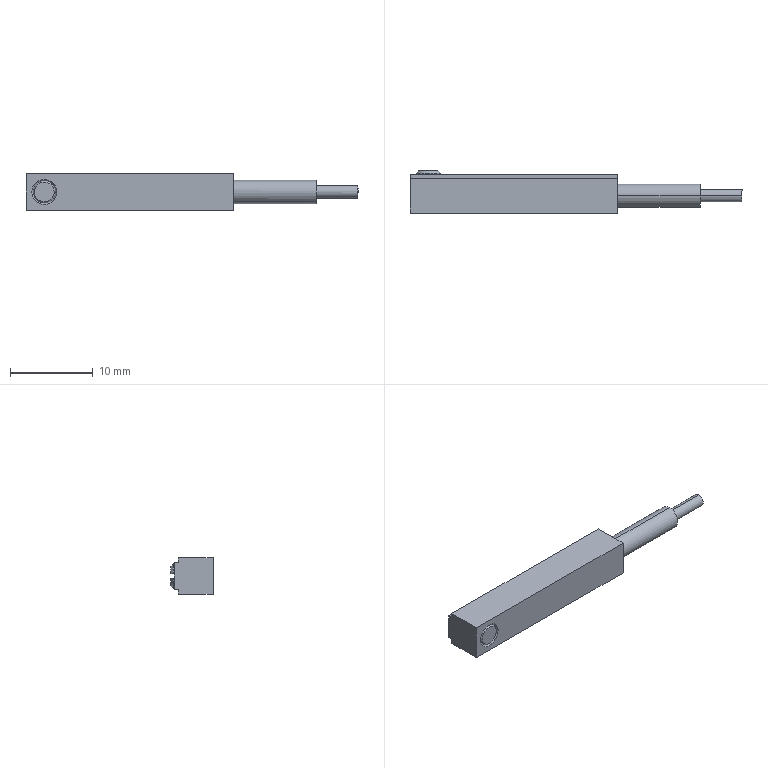Part | SolidWorks | features BaseBody 1 | 1 solid | 34 faces | box 40 x 5.1 x 4.4 mm | volume 573.817 mm3 | plane 20 | cylinder 7 | cone 7 | commonest cylinder face diameters 3 x3 1.5 x2 2.8 x2
STEP:
#1=CARTESIAN_POINT('',(35.,0.,-0.75));
#2=VERTEX_POINT('',#1);
#3=CARTESIAN_POINT('',(35.,0.,0.75));
#4=VERTEX_POINT('',#3);
#5=CARTESIAN_POINT('',(35.,0.,-0.75));
#6=CARTESIAN_POINT('',(35.,0.1963,-0.75));
#7=CARTESIAN_POINT('',(35.,0.3915,-0.6692));
#8=CARTESIAN_POINT('',(35.,0.6692,-0.3915));
#9=CARTESIAN_POINT('',(35.,0.75,-0.1963));
#10=CARTESIAN_POINT('',(35.,0.75,0.1963));
#11=CARTESIAN_POINT('',(35.,0.6692,0.3915));
#12=CARTESIAN_POINT('',(35.,0.3915,0.6692));
#13=CARTESIAN_POINT('',(35.,0.1963,0.75));
#14=CARTESIAN_POINT('',(35.,0.,0.75));
#15=B_SPLINE_CURVE_WITH_KNOTS('',3,(#5,#6,#7,#8,#9,#10,#11,#12,#13,#14),.UNSPECIFIED.,.F.,.F.,(4,2,2,2,4),(0.,0.7854,1.571,2.356,3.142),.UNSPECIFIED.);
#16=EDGE_CURVE('',#2,#4,#15,.T.);
#17=ORIENTED_EDGE('',*,*,#16,.T.);
#18=CARTESIAN_POINT('',(40.,0.,0.75));
#19=VERTEX_POINT('',#18);
#20=CARTESIAN_POINT('',(40.,0.,0.75));
#21=DIRECTION('',(1.,0.,0.));
#22=VECTOR('',#21,1000.);
#23=LINE('',#20,#22);
#24=EDGE_CURVE('',#4,#19,#23,.T.);
#25=ORIENTED_EDGE('',*,*,#24,.T.);
#26=CARTESIAN_POINT('',(40.,0.,-0.75));
#27=VERTEX_POINT('',#26);
#28=CARTESIAN_POINT('',(40.,0.,-0.75));
#29=CARTESIAN_POINT('',(40.,0.1989,-0.75));
#30=CARTESIAN_POINT('',(40.,0.3897,-0.671));
#31=CARTESIAN_POINT('',(40.,0.671,-0.3897));
#32=CARTESIAN_POINT('',(40.,0.75,-0.1989));
#33=CARTESIAN_POINT('',(40.,0.75,0.1989));
#34=CARTESIAN_POINT('',(40.,0.671,0.3897));
#35=CARTESIAN_POINT('',(40.,0.3897,0.671));
#36=CARTESIAN_POINT('',(40.,0.1989,0.75));
#37=CARTESIAN_POINT('',(40.,0.,0.75));
#38=B_SPLINE_CURVE_WITH_KNOTS('',3,(#28,#29,#30,#31,#32,#33,#34,#35,#36,#37),.UNSPECIFIED.,.F.,.F.,(4,2,2,2,4),(0.,0.7854,1.571,2.356,3.142),.UNSPECIFIED.);
#39=EDGE_CURVE('',#27,#19,#38,.T.);
#40=ORIENTED_EDGE('',*,*,#39,.F.);
#41=CARTESIAN_POINT('',(40.,0.,-0.75));
#42=DIRECTION('',(1.,0.,0.));
#43=VECTOR('',#42,1000.);
#44=LINE('',#41,#43);
#45=EDGE_CURVE('',#2,#27,#44,.T.);
#46=ORIENTED_EDGE('',*,*,#45,.F.);
#47=EDGE_LOOP('',(#17,#25,#40,#46));
#48=FACE_OUTER_BOUND('',#47,.T.);
#49=CARTESIAN_POINT('',(40.,0.,0.));
#50=DIRECTION('',(1.,0.,0.));
#51=DIRECTION('',(0.,0.,-1.));
#52=AXIS2_PLACEMENT_3D('',#49,#50,#51);
#53=CYLINDRICAL_SURFACE('',#52,0.75);
#54=ADVANCED_FACE('',(#48),#53,.T.);
#55=CARTESIAN_POINT('',(25.,0.,-1.4));
#56=VERTEX_POINT('',#55);
#57=CARTESIAN_POINT('',(25.,0.,1.4));
#58=VERTEX_POINT('',#57);
#59=CARTESIAN_POINT('',(25.,0.,-1.4));
#60=CARTESIAN_POINT('',(25.,0.1833,-1.4));
#61=CARTESIAN_POINT('',(25.,0.3664,-1.364));
#62=CARTESIAN_POINT('',(25.,0.7051,-1.223));
#63=CARTESIAN_POINT('',(25.,0.8604,-1.12));
#64=CARTESIAN_POINT('',(25.,1.12,-0.8604));
#65=CARTESIAN_POINT('',(25.,1.223,-0.7051));
#66=CARTESIAN_POINT('',(25.,1.364,-0.3664));
#67=CARTESIAN_POINT('',(25.,1.4,-0.1833));
#68=CARTESIAN_POINT('',(25.,1.4,0.1833));
#69=CARTESIAN_POINT('',(25.,1.364,0.3664));
#70=CARTESIAN_POINT('',(25.,1.223,0.7051));
#71=CARTESIAN_POINT('',(25.,1.12,0.8604));
#72=CARTESIAN_POINT('',(25.,0.8604,1.12));
#73=CARTESIAN_POINT('',(25.,0.7051,1.223));
#74=CARTESIAN_POINT('',(25.,0.3664,1.364));
#75=CARTESIAN_POINT('',(25.,0.1833,1.4));
#76=CARTESIAN_POINT('',(25.,0.,1.4));
#77=B_SPLINE_CURVE_WITH_KNOTS('',3,(#59,#60,#61,#62,#63,#64,#65,#66,#67,#68,#69,#70,#71,#72,#73,#74,#75,#76),.UNSPECIFIED.,.F.,.F.,(4,2,2,2,2,2,2,2,4),(0.,0.3927,0.7854,1.178,1.571,1.963,2.356,2.749,3.142),.UNSPECIFIED.);
#78=EDGE_CURVE('',#56,#58,#77,.T.);
#79=ORIENTED_EDGE('',*,*,#78,.T.);
#80=CARTESIAN_POINT('',(35.,0.,1.4));
#81=VERTEX_POINT('',#80);
#82=CARTESIAN_POINT('',(40.,0.,1.4));
#83=DIRECTION('',(1.,0.,0.));
#84=VECTOR('',#83,1000.);
#85=LINE('',#82,#84);
#86=EDGE_CURVE('',#58,#81,#85,.T.);
#87=ORIENTED_EDGE('',*,*,#86,.T.);
#88=CARTESIAN_POINT('',(35.,0.,-1.4));
#89=VERTEX_POINT('',#88);
#90=CARTESIAN_POINT('',(35.,0.,-1.4));
#91=CARTESIAN_POINT('',(35.,0.1857,-1.4));
#92=CARTESIAN_POINT('',(35.,0.3642,-1.364));
#93=CARTESIAN_POINT('',(35.,0.7073,-1.222));
#94=CARTESIAN_POINT('',(35.,0.8587,-1.121));
#95=CARTESIAN_POINT('',(35.,1.121,-0.8587));
#96=CARTESIAN_POINT('',(35.,1.222,-0.7073));
#97=CARTESIAN_POINT('',(35.,1.364,-0.3642));
#98=CARTESIAN_POINT('',(35.,1.4,-0.1857));
#99=CARTESIAN_POINT('',(35.,1.4,0.1857));
#100=CARTESIAN_POINT('',(35.,1.364,0.3642));
#101=CARTESIAN_POINT('',(35.,1.222,0.7073));
#102=CARTESIAN_POINT('',(35.,1.121,0.8587));
#103=CARTESIAN_POINT('',(35.,0.8587,1.121));
#104=CARTESIAN_POINT('',(35.,0.7073,1.222));
#105=CARTESIAN_POINT('',(35.,0.3642,1.364));
#106=CARTESIAN_POINT('',(35.,0.1857,1.4));
#107=CARTESIAN_POINT('',(35.,0.,1.4));
#108=B_SPLINE_CURVE_WITH_KNOTS('',3,(#90,#91,#92,#93,#94,#95,#96,#97,#98,#99,#100,#101,#102,#103,#104,#105,#106,#107),.UNSPECIFIED.,.F.,.F.,(4,2,2,2,2,2,2,2,4),(0.,0.3927,0.7854,1.178,1.571,1.963,2.356,2.749,3.142),.UNSPECIFIED.);
#109=EDGE_CURVE('',#89,#81,#108,.T.);
#110=ORIENTED_EDGE('',*,*,#109,.F.);
#111=CARTESIAN_POINT('',(40.,0.,-1.4));
#112=DIRECTION('',(1.,0.,0.));
#113=VECTOR('',#112,1000.);
#114=LINE('',#111,#113);
#115=EDGE_CURVE('',#56,#89,#114,.T.);
#116=ORIENTED_EDGE('',*,*,#115,.F.);
#117=EDGE_LOOP('',(#79,#87,#110,#116));
#118=FACE_OUTER_BOUND('',#117,.T.);
#119=CARTESIAN_POINT('',(40.,0.,0.));
#120=DIRECTION('',(1.,0.,0.));
#121=DIRECTION('',(0.,0.,-1.));
#122=AXIS2_PLACEMENT_3D('',#119,#120,#121);
#123=CYLINDRICAL_SURFACE('',#122,1.4);
#124=ADVANCED_FACE('',(#118),#123,.T.);
#125=CARTESIAN_POINT('',(2.2,-2.1,-1.194));
#126=VERTEX_POINT('',#125);
#127=CARTESIAN_POINT('',(2.2,-2.1,1.194));
#128=VERTEX_POINT('',#127);
#129=CARTESIAN_POINT('',(2.2,-2.1,-1.194));
#130=CARTESIAN_POINT('',(2.358,-2.1,-1.194));
#131=CARTESIAN_POINT('',(2.511,-2.1,-1.163));
#132=CARTESIAN_POINT('',(2.803,-2.1,-1.042));
#133=CARTESIAN_POINT('',(2.932,-2.1,-0.9558));
#134=CARTESIAN_POINT('',(3.156,-2.1,-0.732));
#135=CARTESIAN_POINT('',(3.242,-2.1,-0.603));
#136=CARTESIAN_POINT('',(3.363,-2.1,-0.3105));
#137=CARTESIAN_POINT('',(3.394,-2.1,-0.1583));
#138=CARTESIAN_POINT('',(3.394,-2.1,0.1583));
#139=CARTESIAN_POINT('',(3.363,-2.1,0.3105));
#140=CARTESIAN_POINT('',(3.242,-2.1,0.603));
#141=CARTESIAN_POINT('',(3.156,-2.1,0.732));
#142=CARTESIAN_POINT('',(2.932,-2.1,0.9558));
#143=CARTESIAN_POINT('',(2.803,-2.1,1.042));
#144=CARTESIAN_POINT('',(2.511,-2.1,1.163));
#145=CARTESIAN_POINT('',(2.358,-2.1,1.194));
#146=CARTESIAN_POINT('',(2.2,-2.1,1.194));
#147=B_SPLINE_CURVE_WITH_KNOTS('',3,(#129,#130,#131,#132,#133,#134,#135,#136,#137,#138,#139,#140,#141,#142,#143,#144,#145,#146),.UNSPECIFIED.,.F.,.F.,(4,2,2,2,2,2,2,2,4),(0.,0.3927,0.7854,1.178,1.571,1.963,2.356,2.749,3.142),.UNSPECIFIED.);
#148=EDGE_CURVE('',#126,#128,#147,.T.);
#149=ORIENTED_EDGE('',*,*,#148,.F.);
#150=CARTESIAN_POINT('',(2.2,-1.947,-1.347));
#151=VERTEX_POINT('',#150);
#152=CARTESIAN_POINT('',(2.2,-1.793,-1.5));
#153=DIRECTION('',(0.,0.7071,-0.7071));
#154=VECTOR('',#153,1000.);
#155=LINE('',#152,#154);
#156=EDGE_CURVE('',#126,#151,#155,.T.);
#157=ORIENTED_EDGE('',*,*,#156,.T.);
#158=CARTESIAN_POINT('',(2.2,-1.947,1.347));
#159=VERTEX_POINT('',#158);
#160=CARTESIAN_POINT('',(2.2,-1.947,1.347));
#161=CARTESIAN_POINT('',(2.376,-1.947,1.347));
#162=CARTESIAN_POINT('',(2.553,-1.947,1.312));
#163=CARTESIAN_POINT('',(2.878,-1.947,1.177));
#164=CARTESIAN_POINT('',(3.028,-1.947,1.077));
#165=CARTESIAN_POINT('',(3.277,-1.947,0.8276));
#166=CARTESIAN_POINT('',(3.377,-1.947,0.6782));
#167=CARTESIAN_POINT('',(3.512,-1.947,0.3525));
#168=CARTESIAN_POINT('',(3.547,-1.947,0.1763));
#169=CARTESIAN_POINT('',(3.547,-1.947,-0.1763));
#170=CARTESIAN_POINT('',(3.512,-1.947,-0.3525));
#171=CARTESIAN_POINT('',(3.377,-1.947,-0.6782));
#172=CARTESIAN_POINT('',(3.277,-1.947,-0.8276));
#173=CARTESIAN_POINT('',(3.028,-1.947,-1.077));
#174=CARTESIAN_POINT('',(2.878,-1.947,-1.177));
#175=CARTESIAN_POINT('',(2.553,-1.947,-1.312));
#176=CARTESIAN_POINT('',(2.376,-1.947,-1.347));
#177=CARTESIAN_POINT('',(2.2,-1.947,-1.347));
#178=B_SPLINE_CURVE_WITH_KNOTS('',3,(#160,#161,#162,#163,#164,#165,#166,#167,#168,#169,#170,#171,#172,#173,#174,#175,#176,#177),.UNSPECIFIED.,.F.,.F.,(4,2,2,2,2,2,2,2,4),(0.,0.3927,0.7854,1.178,1.571,1.963,2.356,2.749,3.142),.UNSPECIFIED.);
#179=EDGE_CURVE('',#159,#151,#178,.T.);
#180=ORIENTED_EDGE('',*,*,#179,.F.);
#181=CARTESIAN_POINT('',(2.2,-1.793,1.5));
#182=DIRECTION('',(0.,0.7071,0.7071));
#183=VECTOR('',#182,1000.);
#184=LINE('',#181,#183);
#185=EDGE_CURVE('',#128,#159,#184,.T.);
#186=ORIENTED_EDGE('',*,*,#185,.F.);
#187=EDGE_LOOP('',(#149,#157,#180,#186));
#188=FACE_OUTER_BOUND('',#187,.T.);
#189=CARTESIAN_POINT('',(2.2,-1.793,0.));
#190=DIRECTION('',(0.,1.,0.));
#191=DIRECTION('',(0.,0.,1.));
#192=AXIS2_PLACEMENT_3D('',#189,#190,#191);
#193=CONICAL_SURFACE('',#192,1.5,0.7854);
#194=ADVANCED_FACE('',(#188),#193,.T.);
#195=CARTESIAN_POINT('',(2.2,-1.947,-1.347));
#196=CARTESIAN_POINT('',(2.024,-1.947,-1.347));
#197=CARTESIAN_POINT('',(1.847,-1.947,-1.312));
#198=CARTESIAN_POINT('',(1.522,-1.947,-1.177));
#199=CARTESIAN_POINT('',(1.372,-1.947,-1.077));
#200=CARTESIAN_POINT('',(1.123,-1.947,-0.8276));
#201=CARTESIAN_POINT('',(1.023,-1.947,-0.6782));
#202=CARTESIAN_POINT('',(0.8883,-1.947,-0.3525));
#203=CARTESIAN_POINT('',(0.8532,-1.947,-0.1763));
#204=CARTESIAN_POINT('',(0.8533,-1.947,0.1763));
#205=CARTESIAN_POINT('',(0.8883,-1.947,0.3525));
#206=CARTESIAN_POINT('',(1.023,-1.947,0.6782));
#207=CARTESIAN_POINT('',(1.123,-1.947,0.8276));
#208=CARTESIAN_POINT('',(1.372,-1.947,1.077));
#209=CARTESIAN_POINT('',(1.522,-1.947,1.177));
#210=CARTESIAN_POINT('',(1.847,-1.947,1.312));
#211=CARTESIAN_POINT('',(2.024,-1.947,1.347));
#212=CARTESIAN_POINT('',(2.2,-1.947,1.347));
#213=B_SPLINE_CURVE_WITH_KNOTS('',3,(#195,#196,#197,#198,#199,#200,#201,#202,#203,#204,#205,#206,#207,#208,#209,#210,#211,#212),.UNSPECIFIED.,.F.,.F.,(4,2,2,2,2,2,2,2,4),(3.142,3.534,3.927,4.32,4.712,5.105,5.498,5.89,6.283),.UNSPECIFIED.);
#214=EDGE_CURVE('',#151,#159,#213,.T.);
#215=ORIENTED_EDGE('',*,*,#214,.T.);
#216=CARTESIAN_POINT('',(2.2,-2.1,1.5));
#217=VERTEX_POINT('',#216);
#218=CARTESIAN_POINT('',(2.2,-1.829,1.229));
#219=DIRECTION('',(0.,-0.7071,0.7071));
#220=VECTOR('',#219,1000.);
#221=LINE('',#218,#220);
#222=EDGE_CURVE('',#159,#217,#221,.T.);
#223=ORIENTED_EDGE('',*,*,#222,.T.);
#224=CARTESIAN_POINT('',(2.2,-2.1,-1.5));
#225=VERTEX_POINT('',#224);
#226=CARTESIAN_POINT('',(2.2,-2.1,1.5));
#227=CARTESIAN_POINT('',(2.004,-2.1,1.5));
#228=CARTESIAN_POINT('',(1.807,-2.1,1.461));
#229=CARTESIAN_POINT('',(1.445,-2.1,1.311));
#230=CARTESIAN_POINT('',(1.278,-2.1,1.2));
#231=CARTESIAN_POINT('',(1.,-2.1,0.9218));
#232=CARTESIAN_POINT('',(0.8893,-2.1,0.7554));
#233=CARTESIAN_POINT('',(0.739,-2.1,0.3926));
#234=CARTESIAN_POINT('',(0.7,-2.1,0.1963));
#235=CARTESIAN_POINT('',(0.7,-2.1,-0.1963));
#236=CARTESIAN_POINT('',(0.739,-2.1,-0.3926));
#237=CARTESIAN_POINT('',(0.8893,-2.1,-0.7554));
#238=CARTESIAN_POINT('',(1.,-2.1,-0.9218));
#239=CARTESIAN_POINT('',(1.278,-2.1,-1.2));
#240=CARTESIAN_POINT('',(1.445,-2.1,-1.311));
#241=CARTESIAN_POINT('',(1.807,-2.1,-1.461));
#242=CARTESIAN_POINT('',(2.004,-2.1,-1.5));
#243=CARTESIAN_POINT('',(2.2,-2.1,-1.5));
#244=B_SPLINE_CURVE_WITH_KNOTS('',3,(#226,#227,#228,#229,#230,#231,#232,#233,#234,#235,#236,#237,#238,#239,#240,#241,#242,#243),.UNSPECIFIED.,.F.,.F.,(4,2,2,2,2,2,2,2,4),(3.142,3.534,3.927,4.32,4.712,5.105,5.498,5.89,6.283),.UNSPECIFIED.);
#245=EDGE_CURVE('',#217,#225,#244,.T.);
#246=ORIENTED_EDGE('',*,*,#245,.T.);
#247=CARTESIAN_POINT('',(2.2,-1.829,-1.229));
#248=DIRECTION('',(0.,-0.7071,-0.7071));
#249=VECTOR('',#248,1000.);
#250=LINE('',#247,#249);
#251=EDGE_CURVE('',#151,#225,#250,.T.);
#252=ORIENTED_EDGE('',*,*,#251,.F.);
#253=EDGE_LOOP('',(#215,#223,#246,#252));
#254=FACE_OUTER_BOUND('',#253,.T.);
#255=CARTESIAN_POINT('',(2.2,-1.829,0.));
#256=DIRECTION('',(0.,-1.,0.));
#257=DIRECTION('',(0.,0.,-1.));
#258=AXIS2_PLACEMENT_3D('',#255,#256,#257);
#259=CONICAL_SURFACE('',#258,1.229,0.7854);
#260=ADVANCED_FACE('',(#254),#259,.F.);
#261=CARTESIAN_POINT('',(0.7303,2.694,-0.3));
#262=VERTEX_POINT('',#261);
#263=CARTESIAN_POINT('',(2.2,2.693,-1.5));
#264=VERTEX_POINT('',#263);
#265=CARTESIAN_POINT('',(2.2,2.693,0.));
#266=DIRECTION('',(0.,-1.,0.));
#267=DIRECTION('',(-0.9798,0.,-0.2));
#268=AXIS2_PLACEMENT_3D('',#265,#266,#267);
#269=CIRCLE('',#268,1.5);
#270=EDGE_CURVE('',#262,#264,#269,.T.);
#271=ORIENTED_EDGE('',*,*,#270,.T.);
#272=CARTESIAN_POINT('',(2.2,2.6,-1.5));
#273=VERTEX_POINT('',#272);
#274=CARTESIAN_POINT('',(2.2,-2.1,-1.5));
#275=DIRECTION('',(0.,-1.,0.));
#276=VECTOR('',#275,1000.);
#277=LINE('',#274,#276);
#278=EDGE_CURVE('',#264,#273,#277,.T.);
#279=ORIENTED_EDGE('',*,*,#278,.T.);
#280=CARTESIAN_POINT('',(0.7303,2.6,-0.3));
#281=VERTEX_POINT('',#280);
#282=CARTESIAN_POINT('',(2.2,2.6,0.));
#283=DIRECTION('',(0.,-1.,0.));
#284=DIRECTION('',(-0.9798,0.,-0.2));
#285=AXIS2_PLACEMENT_3D('',#282,#283,#284);
#286=CIRCLE('',#285,1.5);
#287=EDGE_CURVE('',#281,#273,#286,.T.);
#288=ORIENTED_EDGE('',*,*,#287,.F.);
#289=CARTESIAN_POINT('',(0.7303,2.693,-0.3));
#290=DIRECTION('',(0.,-1.,0.));
#291=VECTOR('',#290,1000.);
#292=LINE('',#289,#291);
#293=EDGE_CURVE('',#262,#281,#292,.T.);
#294=ORIENTED_EDGE('',*,*,#293,.F.);
#295=EDGE_LOOP('',(#271,#279,#288,#294));
#296=FACE_OUTER_BOUND('',#295,.T.);
#297=CARTESIAN_POINT('',(2.2,-2.1,0.));
#298=DIRECTION('',(0.,-1.,0.));
#299=DIRECTION('',(0.,0.,-1.));
#300=AXIS2_PLACEMENT_3D('',#297,#298,#299);
#301=CYLINDRICAL_SURFACE('',#300,1.5);
#302=ADVANCED_FACE('',(#296),#301,.T.);
#303=CARTESIAN_POINT('',(1.045,3.,-0.3));
#304=VERTEX_POINT('',#303);
#305=CARTESIAN_POINT('',(2.2,3.,-1.194));
#306=VERTEX_POINT('',#305);
#307=CARTESIAN_POINT('',(2.2,3.,0.));
#308=DIRECTION('',(0.,-1.,0.));
#309=DIRECTION('',(-0.9679,0.,-0.2514));
#310=AXIS2_PLACEMENT_3D('',#307,#308,#309);
#311=CIRCLE('',#310,1.194);
#312=EDGE_CURVE('',#304,#306,#311,.T.);
#313=ORIENTED_EDGE('',*,*,#312,.T.);
#314=CARTESIAN_POINT('',(2.2,3.,-1.194));
#315=DIRECTION('',(0.,-0.7071,-0.7071));
#316=VECTOR('',#315,1000.);
#317=LINE('',#314,#316);
#318=EDGE_CURVE('',#306,#264,#317,.T.);
#319=ORIENTED_EDGE('',*,*,#318,.T.);
#320=ORIENTED_EDGE('',*,*,#270,.F.);
#321=CARTESIAN_POINT('',(1.045,3.,-0.3));
#322=CARTESIAN_POINT('',(0.9396,2.898,-0.3));
#323=CARTESIAN_POINT('',(0.8349,2.796,-0.3));
#324=CARTESIAN_POINT('',(0.7303,2.694,-0.3));
#325=B_SPLINE_CURVE_WITH_KNOTS('',3,(#321,#322,#323,#324),.UNSPECIFIED.,.F.,.F.,(4,4),(3.343,3.769),.UNSPECIFIED.);
#326=EDGE_CURVE('',#304,#262,#325,.T.);
#327=ORIENTED_EDGE('',*,*,#326,.F.);
#328=EDGE_LOOP('',(#313,#319,#320,#327));
#329=FACE_OUTER_BOUND('',#328,.T.);
#330=CARTESIAN_POINT('',(2.2,3.,0.));
#331=DIRECTION('',(0.,-1.,0.));
#332=DIRECTION('',(0.,0.,-1.));
#333=AXIS2_PLACEMENT_3D('',#330,#331,#332);
#334=CONICAL_SURFACE('',#333,1.194,0.7854);
#335=ADVANCED_FACE('',(#329),#334,.T.);
#336=CARTESIAN_POINT('',(0.,2.6,-1.6));
#337=VERTEX_POINT('',#336);
#338=CARTESIAN_POINT('',(0.,2.6,1.6));
#339=VERTEX_POINT('',#338);
#340=CARTESIAN_POINT('',(0.,2.6,-1.6));
#341=DIRECTION('',(0.,0.,1.));
#342=VECTOR('',#341,1000.);
#343=LINE('',#340,#342);
#344=EDGE_CURVE('',#337,#339,#343,.T.);
#345=ORIENTED_EDGE('',*,*,#344,.T.);
#346=CARTESIAN_POINT('',(25.,2.6,1.6));
#347=VERTEX_POINT('',#346);
#348=CARTESIAN_POINT('',(25.,2.6,1.6));
#349=DIRECTION('',(-1.,0.,0.));
#350=VECTOR('',#349,1000.);
#351=LINE('',#348,#350);
#352=EDGE_CURVE('',#347,#339,#351,.T.);
#353=ORIENTED_EDGE('',*,*,#352,.F.);
#354=CARTESIAN_POINT('',(25.,2.6,-1.6));
#355=VERTEX_POINT('',#354);
#356=CARTESIAN_POINT('',(25.,2.6,-1.6));
#357=DIRECTION('',(0.,0.,1.));
#358=VECTOR('',#357,1000.);
#359=LINE('',#356,#358);
#360=EDGE_CURVE('',#355,#347,#359,.T.);
#361=ORIENTED_EDGE('',*,*,#360,.F.);
#362=CARTESIAN_POINT('',(25.,2.6,-1.6));
#363=DIRECTION('',(-1.,0.,0.));
#364=VECTOR('',#363,1000.);
#365=LINE('',#362,#364);
#366=EDGE_CURVE('',#355,#337,#365,.T.);
#367=ORIENTED_EDGE('',*,*,#366,.T.);
#368=EDGE_LOOP('',(#345,#353,#361,#367));
#369=FACE_OUTER_BOUND('',#368,.T.);
#370=CARTESIAN_POINT('',(3.7,2.6,0.3));
#371=VERTEX_POINT('',#370);
#372=CARTESIAN_POINT('',(3.7,2.6,-0.3));
#373=VERTEX_POINT('',#372);
#374=CARTESIAN_POINT('',(3.7,2.6,0.3));
#375=DIRECTION('',(0.,0.,-1.));
#376=VECTOR('',#375,1000.);
#377=LINE('',#374,#376);
#378=EDGE_CURVE('',#371,#373,#377,.T.);
#379=ORIENTED_EDGE('',*,*,#378,.F.);
#380=CARTESIAN_POINT('',(3.67,2.6,0.3));
#381=VERTEX_POINT('',#380);
#382=CARTESIAN_POINT('',(3.7,2.6,0.3));
#383=DIRECTION('',(-1.,0.,0.));
#384=VECTOR('',#383,1000.);
#385=LINE('',#382,#384);
#386=EDGE_CURVE('',#371,#381,#385,.T.);
#387=ORIENTED_EDGE('',*,*,#386,.T.);
#388=CARTESIAN_POINT('',(0.7303,2.6,0.3));
#389=VERTEX_POINT('',#388);
#390=CARTESIAN_POINT('',(2.2,2.6,0.));
#391=DIRECTION('',(0.,-1.,0.));
#392=DIRECTION('',(0.9798,0.,0.2));
#393=AXIS2_PLACEMENT_3D('',#390,#391,#392);
#394=CIRCLE('',#393,1.5);
#395=EDGE_CURVE('',#381,#389,#394,.T.);
#396=ORIENTED_EDGE('',*,*,#395,.T.);
#397=CARTESIAN_POINT('',(0.7,2.6,0.3));
#398=VERTEX_POINT('',#397);
#399=CARTESIAN_POINT('',(0.7303,2.6,0.3));
#400=DIRECTION('',(-1.,0.,0.));
#401=VECTOR('',#400,1000.);
#402=LINE('',#399,#401);
#403=EDGE_CURVE('',#389,#398,#402,.T.);
#404=ORIENTED_EDGE('',*,*,#403,.T.);
#405=CARTESIAN_POINT('',(0.7,2.6,-0.3));
#406=VERTEX_POINT('',#405);
#407=CARTESIAN_POINT('',(0.7,2.6,-0.3));
#408=DIRECTION('',(0.,0.,1.));
#409=VECTOR('',#408,1000.);
#410=LINE('',#407,#409);
#411=EDGE_CURVE('',#406,#398,#410,.T.);
#412=ORIENTED_EDGE('',*,*,#411,.F.);
#413=CARTESIAN_POINT('',(0.7303,2.6,-0.3));
#414=DIRECTION('',(-1.,0.,0.));
#415=VECTOR('',#414,1000.);
#416=LINE('',#413,#415);
#417=EDGE_CURVE('',#281,#406,#416,.T.);
#418=ORIENTED_EDGE('',*,*,#417,.F.);
#419=ORIENTED_EDGE('',*,*,#287,.T.);
#420=CARTESIAN_POINT('',(3.67,2.6,-0.3));
#421=VERTEX_POINT('',#420);
#422=CARTESIAN_POINT('',(2.2,2.6,0.));
#423=DIRECTION('',(0.,-1.,0.));
#424=DIRECTION('',(-0.9798,0.,-0.2));
#425=AXIS2_PLACEMENT_3D('',#422,#423,#424);
#426=CIRCLE('',#425,1.5);
#427=EDGE_CURVE('',#273,#421,#426,.T.);
#428=ORIENTED_EDGE('',*,*,#427,.T.);
#429=CARTESIAN_POINT('',(3.7,2.6,-0.3));
#430=DIRECTION('',(-1.,0.,0.));
#431=VECTOR('',#430,1000.);
#432=LINE('',#429,#431);
#433=EDGE_CURVE('',#373,#421,#432,.T.);
#434=ORIENTED_EDGE('',*,*,#433,.F.);
#435=EDGE_LOOP('',(#379,#387,#396,#404,#412,#418,#419,#428,#434));
#436=FACE_BOUND('',#435,.T.);
#437=CARTESIAN_POINT('',(25.,2.6,-1.6));
#438=DIRECTION('',(0.,-1.,0.));
#439=DIRECTION('',(0.,0.,-1.));
#440=AXIS2_PLACEMENT_3D('',#437,#438,#439);
#441=PLANE('',#440);
#442=ADVANCED_FACE('',(#369,#436),#441,.F.);
#443=CARTESIAN_POINT('',(3.355,3.,-0.3));
#444=VERTEX_POINT('',#443);
#445=CARTESIAN_POINT('',(3.355,3.,-0.3));
#446=DIRECTION('',(-1.,0.,0.));
#447=VECTOR('',#446,1000.);
#448=LINE('',#445,#447);
#449=EDGE_CURVE('',#444,#304,#448,.T.);
#450=ORIENTED_EDGE('',*,*,#449,.F.);
#451=CARTESIAN_POINT('',(2.2,3.,0.));
#452=DIRECTION('',(0.,-1.,0.));
#453=DIRECTION('',(-0.9679,0.,-0.2514));
#454=AXIS2_PLACEMENT_3D('',#451,#452,#453);
#455=CIRCLE('',#454,1.194);
#456=EDGE_CURVE('',#306,#444,#455,.T.);
#457=ORIENTED_EDGE('',*,*,#456,.F.);
#458=ORIENTED_EDGE('',*,*,#312,.F.);
#459=EDGE_LOOP('',(#450,#457,#458));
#460=FACE_OUTER_BOUND('',#459,.T.);
#461=CARTESIAN_POINT('',(2.2,3.,0.));
#462=DIRECTION('',(0.,-1.,0.));
#463=DIRECTION('',(0.,0.,-1.));
#464=AXIS2_PLACEMENT_3D('',#461,#462,#463);
#465=PLANE('',#464);
#466=ADVANCED_FACE('',(#460),#465,.F.);
#467=ORIENTED_EDGE('',*,*,#318,.F.);
#468=ORIENTED_EDGE('',*,*,#456,.T.);
#469=CARTESIAN_POINT('',(3.67,2.694,-0.3));
#470=VERTEX_POINT('',#469);
#471=CARTESIAN_POINT('',(3.67,2.694,-0.3));
#472=CARTESIAN_POINT('',(3.565,2.796,-0.3));
#473=CARTESIAN_POINT('',(3.46,2.898,-0.3));
#474=CARTESIAN_POINT('',(3.355,3.,-0.3));
#475=B_SPLINE_CURVE_WITH_KNOTS('',3,(#471,#472,#473,#474),.UNSPECIFIED.,.F.,.F.,(4,4),(0.0009988,0.4388),.UNSPECIFIED.);
#476=EDGE_CURVE('',#470,#444,#475,.T.);
#477=ORIENTED_EDGE('',*,*,#476,.F.);
#478=CARTESIAN_POINT('',(2.2,2.693,0.));
#479=DIRECTION('',(0.,-1.,0.));
#480=DIRECTION('',(-0.9798,0.,-0.2));
#481=AXIS2_PLACEMENT_3D('',#478,#479,#480);
#482=CIRCLE('',#481,1.5);
#483=EDGE_CURVE('',#264,#470,#482,.T.);
#484=ORIENTED_EDGE('',*,*,#483,.F.);
#485=EDGE_LOOP('',(#467,#468,#477,#484));
#486=FACE_OUTER_BOUND('',#485,.T.);
#487=CARTESIAN_POINT('',(2.2,3.,0.));
#488=DIRECTION('',(0.,-1.,0.));
#489=DIRECTION('',(0.,0.,-1.));
#490=AXIS2_PLACEMENT_3D('',#487,#488,#489);
#491=CONICAL_SURFACE('',#490,1.194,0.7854);
#492=ADVANCED_FACE('',(#486),#491,.T.);
#493=ORIENTED_EDGE('',*,*,#278,.F.);
#494=ORIENTED_EDGE('',*,*,#483,.T.);
#495=CARTESIAN_POINT('',(3.67,2.6,-0.3));
#496=DIRECTION('',(0.,1.,0.));
#497=VECTOR('',#496,1000.);
#498=LINE('',#495,#497);
#499=EDGE_CURVE('',#421,#470,#498,.T.);
#500=ORIENTED_EDGE('',*,*,#499,.F.);
#501=ORIENTED_EDGE('',*,*,#427,.F.);
#502=EDGE_LOOP('',(#493,#494,#500,#501));
#503=FACE_OUTER_BOUND('',#502,.T.);
#504=CARTESIAN_POINT('',(2.2,-2.1,0.));
#505=DIRECTION('',(0.,-1.,0.));
#506=DIRECTION('',(0.,0.,-1.));
#507=AXIS2_PLACEMENT_3D('',#504,#505,#506);
#508=CYLINDRICAL_SURFACE('',#507,1.5);
#509=ADVANCED_FACE('',(#503),#508,.T.);
#510=CARTESIAN_POINT('',(3.67,2.694,0.3));
#511=VERTEX_POINT('',#510);
#512=CARTESIAN_POINT('',(0.7303,2.694,0.3));
#513=VERTEX_POINT('',#512);
#514=CARTESIAN_POINT('',(2.2,2.693,0.));
#515=DIRECTION('',(0.,-1.,0.));
#516=DIRECTION('',(0.9798,0.,0.2));
#517=AXIS2_PLACEMENT_3D('',#514,#515,#516);
#518=CIRCLE('',#517,1.5);
#519=EDGE_CURVE('',#511,#513,#518,.T.);
#520=ORIENTED_EDGE('',*,*,#519,.T.);
#521=CARTESIAN_POINT('',(0.7303,2.693,0.3));
#522=DIRECTION('',(0.,-1.,0.));
#523=VECTOR('',#522,1000.);
#524=LINE('',#521,#523);
#525=EDGE_CURVE('',#513,#389,#524,.T.);
#526=ORIENTED_EDGE('',*,*,#525,.T.);
#527=ORIENTED_EDGE('',*,*,#395,.F.);
#528=CARTESIAN_POINT('',(3.67,2.6,0.3));
#529=DIRECTION('',(0.,1.,0.));
#530=VECTOR('',#529,1000.);
#531=LINE('',#528,#530);
#532=EDGE_CURVE('',#381,#511,#531,.T.);
#533=ORIENTED_EDGE('',*,*,#532,.T.);
#534=EDGE_LOOP('',(#520,#526,#527,#533));
#535=FACE_OUTER_BOUND('',#534,.T.);
#536=CARTESIAN_POINT('',(2.2,-2.1,0.));
#537=DIRECTION('',(0.,-1.,0.));
#538=DIRECTION('',(0.,0.,-1.));
#539=AXIS2_PLACEMENT_3D('',#536,#537,#538);
#540=CYLINDRICAL_SURFACE('',#539,1.5);
#541=ADVANCED_FACE('',(#535),#540,.T.);
#542=ORIENTED_EDGE('',*,*,#222,.F.);
#543=ORIENTED_EDGE('',*,*,#179,.T.);
#544=ORIENTED_EDGE('',*,*,#251,.T.);
#545=CARTESIAN_POINT('',(2.2,-2.1,-1.5));
#546=CARTESIAN_POINT('',(2.396,-2.1,-1.5));
#547=CARTESIAN_POINT('',(2.593,-2.1,-1.461));
#548=CARTESIAN_POINT('',(2.955,-2.1,-1.311));
#549=CARTESIAN_POINT('',(3.122,-2.1,-1.2));
#550=CARTESIAN_POINT('',(3.4,-2.1,-0.9218));
#551=CARTESIAN_POINT('',(3.511,-2.1,-0.7554));
#552=CARTESIAN_POINT('',(3.661,-2.1,-0.3926));
#553=CARTESIAN_POINT('',(3.7,-2.1,-0.1963));
#554=CARTESIAN_POINT('',(3.7,-2.1,0.1963));
#555=CARTESIAN_POINT('',(3.661,-2.1,0.3926));
#556=CARTESIAN_POINT('',(3.511,-2.1,0.7554));
#557=CARTESIAN_POINT('',(3.4,-2.1,0.9218));
#558=CARTESIAN_POINT('',(3.122,-2.1,1.2));
#559=CARTESIAN_POINT('',(2.955,-2.1,1.311));
#560=CARTESIAN_POINT('',(2.593,-2.1,1.461));
#561=CARTESIAN_POINT('',(2.396,-2.1,1.5));
#562=CARTESIAN_POINT('',(2.2,-2.1,1.5));
#563=B_SPLINE_CURVE_WITH_KNOTS('',3,(#545,#546,#547,#548,#549,#550,#551,#552,#553,#554,#555,#556,#557,#558,#559,#560,#561,#562),.UNSPECIFIED.,.F.,.F.,(4,2,2,2,2,2,2,2,4),(0.,0.3927,0.7854,1.178,1.571,1.963,2.356,2.749,3.142),.UNSPECIFIED.);
#564=EDGE_CURVE('',#225,#217,#563,.T.);
#565=ORIENTED_EDGE('',*,*,#564,.T.);
#566=EDGE_LOOP('',(#542,#543,#544,#565));
#567=FACE_OUTER_BOUND('',#566,.T.);
#568=CARTESIAN_POINT('',(2.2,-1.829,0.));
#569=DIRECTION('',(0.,-1.,0.));
#570=DIRECTION('',(0.,0.,-1.));
#571=AXIS2_PLACEMENT_3D('',#568,#569,#570);
#572=CONICAL_SURFACE('',#571,1.229,0.7854);
#573=ADVANCED_FACE('',(#567),#572,.F.);
#574=CARTESIAN_POINT('',(0.,2.1,2.2));
#575=VERTEX_POINT('',#574);
#576=CARTESIAN_POINT('',(0.,-2.1,2.2));
#577=VERTEX_POINT('',#576);
#578=CARTESIAN_POINT('',(0.,2.1,2.2));
#579=DIRECTION('',(0.,-1.,0.));
#580=VECTOR('',#579,1000.);
#581=LINE('',#578,#580);
#582=EDGE_CURVE('',#575,#577,#581,.T.);
#583=ORIENTED_EDGE('',*,*,#582,.T.);
#584=CARTESIAN_POINT('',(25.,-2.1,2.2));
#585=VERTEX_POINT('',#584);
#586=CARTESIAN_POINT('',(25.,-2.1,2.2));
#587=DIRECTION('',(-1.,0.,0.));
#588=VECTOR('',#587,1000.);
#589=LINE('',#586,#588);
#590=EDGE_CURVE('',#585,#577,#589,.T.);
#591=ORIENTED_EDGE('',*,*,#590,.F.);
#592=CARTESIAN_POINT('',(25.,2.1,2.2));
#593=VERTEX_POINT('',#592);
#594=CARTESIAN_POINT('',(25.,2.1,2.2));
#595=DIRECTION('',(0.,-1.,0.));
#596=VECTOR('',#595,1000.);
#597=LINE('',#594,#596);
#598=EDGE_CURVE('',#593,#585,#597,.T.);
#599=ORIENTED_EDGE('',*,*,#598,.F.);
#600=CARTESIAN_POINT('',(25.,2.1,2.2));
#601=DIRECTION('',(-1.,0.,0.));
#602=VECTOR('',#601,1000.);
#603=LINE('',#600,#602);
#604=EDGE_CURVE('',#593,#575,#603,.T.);
#605=ORIENTED_EDGE('',*,*,#604,.T.);
#606=EDGE_LOOP('',(#583,#591,#599,#605));
#607=FACE_OUTER_BOUND('',#606,.T.);
#608=CARTESIAN_POINT('',(25.,2.1,2.2));
#609=DIRECTION('',(0.,0.,-1.));
#610=DIRECTION('',(-1.,0.,0.));
#611=AXIS2_PLACEMENT_3D('',#608,#609,#610);
#612=PLANE('',#611);
#613=ADVANCED_FACE('',(#607),#612,.F.);
#614=ORIENTED_EDGE('',*,*,#564,.F.);
#615=ORIENTED_EDGE('',*,*,#245,.F.);
#616=EDGE_LOOP('',(#614,#615));
#617=FACE_BOUND('',#616,.T.);
#618=CARTESIAN_POINT('',(0.,-2.1,-2.2));
#619=VERTEX_POINT('',#618);
#620=CARTESIAN_POINT('',(0.,-2.1,2.2));
#621=DIRECTION('',(0.,0.,-1.));
#622=VECTOR('',#621,1000.);
#623=LINE('',#620,#622);
#624=EDGE_CURVE('',#577,#619,#623,.T.);
#625=ORIENTED_EDGE('',*,*,#624,.T.);
#626=CARTESIAN_POINT('',(25.,-2.1,-2.2));
#627=VERTEX_POINT('',#626);
#628=CARTESIAN_POINT('',(25.,-2.1,-2.2));
#629=DIRECTION('',(-1.,0.,0.));
#630=VECTOR('',#629,1000.);
#631=LINE('',#628,#630);
#632=EDGE_CURVE('',#627,#619,#631,.T.);
#633=ORIENTED_EDGE('',*,*,#632,.F.);
#634=CARTESIAN_POINT('',(25.,-2.1,2.2));
#635=DIRECTION('',(0.,0.,-1.));
#636=VECTOR('',#635,1000.);
#637=LINE('',#634,#636);
#638=EDGE_CURVE('',#585,#627,#637,.T.);
#639=ORIENTED_EDGE('',*,*,#638,.F.);
#640=ORIENTED_EDGE('',*,*,#590,.T.);
#641=EDGE_LOOP('',(#625,#633,#639,#640));
#642=FACE_OUTER_BOUND('',#641,.T.);
#643=CARTESIAN_POINT('',(25.,-2.1,2.2));
#644=DIRECTION('',(0.,1.,0.));
#645=DIRECTION('',(0.,0.,1.));
#646=AXIS2_PLACEMENT_3D('',#643,#644,#645);
#647=PLANE('',#646);
#648=ADVANCED_FACE('',(#617,#642),#647,.F.);
#649=CARTESIAN_POINT('',(0.,2.1,-2.2));
#650=VERTEX_POINT('',#649);
#651=CARTESIAN_POINT('',(0.,-2.1,-2.2));
#652=DIRECTION('',(0.,1.,0.));
#653=VECTOR('',#652,1000.);
#654=LINE('',#651,#653);
#655=EDGE_CURVE('',#619,#650,#654,.T.);
#656=ORIENTED_EDGE('',*,*,#655,.T.);
#657=CARTESIAN_POINT('',(25.,2.1,-2.2));
#658=VERTEX_POINT('',#657);
#659=CARTESIAN_POINT('',(25.,2.1,-2.2));
#660=DIRECTION('',(-1.,0.,0.));
#661=VECTOR('',#660,1000.);
#662=LINE('',#659,#661);
#663=EDGE_CURVE('',#658,#650,#662,.T.);
#664=ORIENTED_EDGE('',*,*,#663,.F.);
#665=CARTESIAN_POINT('',(25.,-2.1,-2.2));
#666=DIRECTION('',(0.,1.,0.));
#667=VECTOR('',#666,1000.);
#668=LINE('',#665,#667);
#669=EDGE_CURVE('',#627,#658,#668,.T.);
#670=ORIENTED_EDGE('',*,*,#669,.F.);
#671=ORIENTED_EDGE('',*,*,#632,.T.);
#672=EDGE_LOOP('',(#656,#664,#670,#671));
#673=FACE_OUTER_BOUND('',#672,.T.);
#674=CARTESIAN_POINT('',(25.,-2.1,-2.2));
#675=DIRECTION('',(0.,0.,1.));
#676=DIRECTION('',(1.,0.,0.));
#677=AXIS2_PLACEMENT_3D('',#674,#675,#676);
#678=PLANE('',#677);
#679=ADVANCED_FACE('',(#673),#678,.F.);
#680=CARTESIAN_POINT('',(0.,2.1,-1.6));
#681=VERTEX_POINT('',#680);
#682=CARTESIAN_POINT('',(0.,2.1,-2.2));
#683=DIRECTION('',(0.,0.,1.));
#684=VECTOR('',#683,1000.);
#685=LINE('',#682,#684);
#686=EDGE_CURVE('',#650,#681,#685,.T.);
#687=ORIENTED_EDGE('',*,*,#686,.T.);
#688=CARTESIAN_POINT('',(25.,2.1,-1.6));
#689=VERTEX_POINT('',#688);
#690=CARTESIAN_POINT('',(25.,2.1,-1.6));
#691=DIRECTION('',(-1.,0.,0.));
#692=VECTOR('',#691,1000.);
#693=LINE('',#690,#692);
#694=EDGE_CURVE('',#689,#681,#693,.T.);
#695=ORIENTED_EDGE('',*,*,#694,.F.);
#696=CARTESIAN_POINT('',(25.,2.1,-2.2));
#697=DIRECTION('',(0.,0.,1.));
#698=VECTOR('',#697,1000.);
#699=LINE('',#696,#698);
#700=EDGE_CURVE('',#658,#689,#699,.T.);
#701=ORIENTED_EDGE('',*,*,#700,.F.);
#702=ORIENTED_EDGE('',*,*,#663,.T.);
#703=EDGE_LOOP('',(#687,#695,#701,#702));
#704=FACE_OUTER_BOUND('',#703,.T.);
#705=CARTESIAN_POINT('',(25.,2.1,-2.2));
#706=DIRECTION('',(0.,-1.,0.));
#707=DIRECTION('',(0.,0.,-1.));
#708=AXIS2_PLACEMENT_3D('',#705,#706,#707);
#709=PLANE('',#708);
#710=ADVANCED_FACE('',(#704),#709,.F.);
#711=CARTESIAN_POINT('',(0.,2.1,-1.6));
#712=DIRECTION('',(0.,1.,0.));
#713=VECTOR('',#712,1000.);
#714=LINE('',#711,#713);
#715=EDGE_CURVE('',#681,#337,#714,.T.);
#716=ORIENTED_EDGE('',*,*,#715,.T.);
#717=ORIENTED_EDGE('',*,*,#366,.F.);
#718=CARTESIAN_POINT('',(25.,2.1,-1.6));
#719=DIRECTION('',(0.,1.,0.));
#720=VECTOR('',#719,1000.);
#721=LINE('',#718,#720);
#722=EDGE_CURVE('',#689,#355,#721,.T.);
#723=ORIENTED_EDGE('',*,*,#722,.F.);
#724=ORIENTED_EDGE('',*,*,#694,.T.);
#725=EDGE_LOOP('',(#716,#717,#723,#724));
#726=FACE_OUTER_BOUND('',#725,.T.);
#727=CARTESIAN_POINT('',(25.,2.1,-1.6));
#728=DIRECTION('',(0.,0.,1.));
#729=DIRECTION('',(1.,0.,0.));
#730=AXIS2_PLACEMENT_3D('',#727,#728,#729);
#731=PLANE('',#730);
#732=ADVANCED_FACE('',(#726),#731,.F.);
#733=CARTESIAN_POINT('',(0.,2.1,1.6));
#734=VERTEX_POINT('',#733);
#735=CARTESIAN_POINT('',(0.,2.6,1.6));
#736=DIRECTION('',(0.,-1.,0.));
#737=VECTOR('',#736,1000.);
#738=LINE('',#735,#737);
#739=EDGE_CURVE('',#339,#734,#738,.T.);
#740=ORIENTED_EDGE('',*,*,#739,.T.);
#741=CARTESIAN_POINT('',(25.,2.1,1.6));
#742=VERTEX_POINT('',#741);
#743=CARTESIAN_POINT('',(25.,2.1,1.6));
#744=DIRECTION('',(-1.,0.,0.));
#745=VECTOR('',#744,1000.);
#746=LINE('',#743,#745);
#747=EDGE_CURVE('',#742,#734,#746,.T.);
#748=ORIENTED_EDGE('',*,*,#747,.F.);
#749=CARTESIAN_POINT('',(25.,2.6,1.6));
#750=DIRECTION('',(0.,-1.,0.));
#751=VECTOR('',#750,1000.);
#752=LINE('',#749,#751);
#753=EDGE_CURVE('',#347,#742,#752,.T.);
#754=ORIENTED_EDGE('',*,*,#753,.F.);
#755=ORIENTED_EDGE('',*,*,#352,.T.);
#756=EDGE_LOOP('',(#740,#748,#754,#755));
#757=FACE_OUTER_BOUND('',#756,.T.);
#758=CARTESIAN_POINT('',(25.,2.6,1.6));
#759=DIRECTION('',(0.,0.,-1.));
#760=DIRECTION('',(-1.,0.,0.));
#761=AXIS2_PLACEMENT_3D('',#758,#759,#760);
#762=PLANE('',#761);
#763=ADVANCED_FACE('',(#757),#762,.F.);
#764=CARTESIAN_POINT('',(0.,2.1,1.6));
#765=DIRECTION('',(0.,0.,1.));
#766=VECTOR('',#765,1000.);
#767=LINE('',#764,#766);
#768=EDGE_CURVE('',#734,#575,#767,.T.);
#769=ORIENTED_EDGE('',*,*,#768,.T.);
#770=ORIENTED_EDGE('',*,*,#604,.F.);
#771=CARTESIAN_POINT('',(25.,2.1,1.6));
#772=DIRECTION('',(0.,0.,1.));
#773=VECTOR('',#772,1000.);
#774=LINE('',#771,#773);
#775=EDGE_CURVE('',#742,#593,#774,.T.);
#776=ORIENTED_EDGE('',*,*,#775,.F.);
#777=ORIENTED_EDGE('',*,*,#747,.T.);
#778=EDGE_LOOP('',(#769,#770,#776,#777));
#779=FACE_OUTER_BOUND('',#778,.T.);
#780=CARTESIAN_POINT('',(25.,2.1,1.6));
#781=DIRECTION('',(0.,-1.,0.));
#782=DIRECTION('',(0.,0.,-1.));
#783=AXIS2_PLACEMENT_3D('',#780,#781,#782);
#784=PLANE('',#783);
#785=ADVANCED_FACE('',(#779),#784,.F.);
#786=ORIENTED_EDGE('',*,*,#78,.F.);
#787=CARTESIAN_POINT('',(25.,0.,1.4));
#788=CARTESIAN_POINT('',(25.,-0.1833,1.4));
#789=CARTESIAN_POINT('',(25.,-0.3664,1.364));
#790=CARTESIAN_POINT('',(25.,-0.7051,1.223));
#791=CARTESIAN_POINT('',(25.,-0.8604,1.12));
#792=CARTESIAN_POINT('',(25.,-1.12,0.8604));
#793=CARTESIAN_POINT('',(25.,-1.223,0.7051));
#794=CARTESIAN_POINT('',(25.,-1.364,0.3664));
#795=CARTESIAN_POINT('',(25.,-1.4,0.1833));
#796=CARTESIAN_POINT('',(25.,-1.4,-0.1833));
#797=CARTESIAN_POINT('',(25.,-1.364,-0.3664));
#798=CARTESIAN_POINT('',(25.,-1.223,-0.7051));
#799=CARTESIAN_POINT('',(25.,-1.12,-0.8604));
#800=CARTESIAN_POINT('',(25.,-0.8604,-1.12));
#801=CARTESIAN_POINT('',(25.,-0.7051,-1.223));
#802=CARTESIAN_POINT('',(25.,-0.3664,-1.364));
#803=CARTESIAN_POINT('',(25.,-0.1833,-1.4));
#804=CARTESIAN_POINT('',(25.,0.,-1.4));
#805=B_SPLINE_CURVE_WITH_KNOTS('',3,(#787,#788,#789,#790,#791,#792,#793,#794,#795,#796,#797,#798,#799,#800,#801,#802,#803,#804),.UNSPECIFIED.,.F.,.F.,(4,2,2,2,2,2,2,2,4),(3.142,3.534,3.927,4.32,4.712,5.105,5.498,5.89,6.283),.UNSPECIFIED.);
#806=EDGE_CURVE('',#58,#56,#805,.T.);
#807=ORIENTED_EDGE('',*,*,#806,.F.);
#808=EDGE_LOOP('',(#786,#807));
#809=FACE_BOUND('',#808,.T.);
#810=ORIENTED_EDGE('',*,*,#598,.T.);
#811=ORIENTED_EDGE('',*,*,#638,.T.);
#812=ORIENTED_EDGE('',*,*,#669,.T.);
#813=ORIENTED_EDGE('',*,*,#700,.T.);
#814=ORIENTED_EDGE('',*,*,#722,.T.);
#815=ORIENTED_EDGE('',*,*,#360,.T.);
#816=ORIENTED_EDGE('',*,*,#753,.T.);
#817=ORIENTED_EDGE('',*,*,#775,.T.);
#818=EDGE_LOOP('',(#810,#811,#812,#813,#814,#815,#816,#817));
#819=FACE_OUTER_BOUND('',#818,.T.);
#820=CARTESIAN_POINT('',(25.,0.,0.));
#821=DIRECTION('',(1.,0.,0.));
#822=DIRECTION('',(0.,0.,-1.));
#823=AXIS2_PLACEMENT_3D('',#820,#821,#822);
#824=PLANE('',#823);
#825=ADVANCED_FACE('',(#809,#819),#824,.T.);
#826=ORIENTED_EDGE('',*,*,#582,.F.);
#827=ORIENTED_EDGE('',*,*,#768,.F.);
#828=ORIENTED_EDGE('',*,*,#739,.F.);
#829=ORIENTED_EDGE('',*,*,#344,.F.);
#830=ORIENTED_EDGE('',*,*,#715,.F.);
#831=ORIENTED_EDGE('',*,*,#686,.F.);
#832=ORIENTED_EDGE('',*,*,#655,.F.);
#833=ORIENTED_EDGE('',*,*,#624,.F.);
#834=EDGE_LOOP('',(#826,#827,#828,#829,#830,#831,#832,#833));
#835=FACE_OUTER_BOUND('',#834,.T.);
#836=CARTESIAN_POINT('',(0.,0.,0.));
#837=DIRECTION('',(1.,0.,0.));
#838=DIRECTION('',(0.,0.,-1.));
#839=AXIS2_PLACEMENT_3D('',#836,#837,#838);
#840=PLANE('',#839);
#841=ADVANCED_FACE('',(#835),#840,.F.);
#842=CARTESIAN_POINT('',(2.2,-2.1,1.194));
#843=CARTESIAN_POINT('',(2.042,-2.1,1.194));
#844=CARTESIAN_POINT('',(1.889,-2.1,1.163));
#845=CARTESIAN_POINT('',(1.597,-2.1,1.042));
#846=CARTESIAN_POINT('',(1.468,-2.1,0.9558));
#847=CARTESIAN_POINT('',(1.244,-2.1,0.732));
#848=CARTESIAN_POINT('',(1.158,-2.1,0.603));
#849=CARTESIAN_POINT('',(1.037,-2.1,0.3105));
#850=CARTESIAN_POINT('',(1.007,-2.1,0.1583));
#851=CARTESIAN_POINT('',(1.006,-2.1,-0.1583));
#852=CARTESIAN_POINT('',(1.037,-2.1,-0.3105));
#853=CARTESIAN_POINT('',(1.158,-2.1,-0.603));
#854=CARTESIAN_POINT('',(1.244,-2.1,-0.732));
#855=CARTESIAN_POINT('',(1.468,-2.1,-0.9558));
#856=CARTESIAN_POINT('',(1.597,-2.1,-1.042));
#857=CARTESIAN_POINT('',(1.889,-2.1,-1.163));
#858=CARTESIAN_POINT('',(2.042,-2.1,-1.194));
#859=CARTESIAN_POINT('',(2.2,-2.1,-1.194));
#860=B_SPLINE_CURVE_WITH_KNOTS('',3,(#842,#843,#844,#845,#846,#847,#848,#849,#850,#851,#852,#853,#854,#855,#856,#857,#858,#859),.UNSPECIFIED.,.F.,.F.,(4,2,2,2,2,2,2,2,4),(3.142,3.534,3.927,4.32,4.712,5.105,5.498,5.89,6.283),.UNSPECIFIED.);
#861=EDGE_CURVE('',#128,#126,#860,.T.);
#862=ORIENTED_EDGE('',*,*,#861,.T.);
#863=ORIENTED_EDGE('',*,*,#148,.T.);
#864=EDGE_LOOP('',(#862,#863));
#865=FACE_OUTER_BOUND('',#864,.T.);
#866=CARTESIAN_POINT('',(3.393,-2.1,0.));
#867=DIRECTION('',(0.,1.,0.));
#868=DIRECTION('',(0.,0.,1.));
#869=AXIS2_PLACEMENT_3D('',#866,#867,#868);
#870=PLANE('',#869);
#871=ADVANCED_FACE('',(#865),#870,.F.);
#872=ORIENTED_EDGE('',*,*,#156,.F.);
#873=ORIENTED_EDGE('',*,*,#861,.F.);
#874=ORIENTED_EDGE('',*,*,#185,.T.);
#875=ORIENTED_EDGE('',*,*,#214,.F.);
#876=EDGE_LOOP('',(#872,#873,#874,#875));
#877=FACE_OUTER_BOUND('',#876,.T.);
#878=CARTESIAN_POINT('',(2.2,-1.793,0.));
#879=DIRECTION('',(0.,1.,0.));
#880=DIRECTION('',(0.,0.,1.));
#881=AXIS2_PLACEMENT_3D('',#878,#879,#880);
#882=CONICAL_SURFACE('',#881,1.5,0.7854);
#883=ADVANCED_FACE('',(#877),#882,.T.);
#884=CARTESIAN_POINT('',(3.355,3.,0.3));
#885=VERTEX_POINT('',#884);
#886=CARTESIAN_POINT('',(1.045,3.,0.3));
#887=VERTEX_POINT('',#886);
#888=CARTESIAN_POINT('',(2.2,3.,0.));
#889=DIRECTION('',(0.,-1.,0.));
#890=DIRECTION('',(0.9679,0.,0.2514));
#891=AXIS2_PLACEMENT_3D('',#888,#889,#890);
#892=CIRCLE('',#891,1.193);
#893=EDGE_CURVE('',#885,#887,#892,.T.);
#894=ORIENTED_EDGE('',*,*,#893,.F.);
#895=CARTESIAN_POINT('',(3.355,3.,0.3));
#896=DIRECTION('',(-1.,0.,0.));
#897=VECTOR('',#896,1000.);
#898=LINE('',#895,#897);
#899=EDGE_CURVE('',#885,#887,#898,.T.);
#900=ORIENTED_EDGE('',*,*,#899,.T.);
#901=EDGE_LOOP('',(#894,#900));
#902=FACE_OUTER_BOUND('',#901,.T.);
#903=CARTESIAN_POINT('',(2.2,3.,0.));
#904=DIRECTION('',(0.,-1.,0.));
#905=DIRECTION('',(0.,0.,-1.));
#906=AXIS2_PLACEMENT_3D('',#903,#904,#905);
#907=PLANE('',#906);
#908=ADVANCED_FACE('',(#902),#907,.F.);
#909=ORIENTED_EDGE('',*,*,#519,.F.);
#910=CARTESIAN_POINT('',(3.67,2.694,0.3));
#911=CARTESIAN_POINT('',(3.565,2.796,0.3));
#912=CARTESIAN_POINT('',(3.46,2.899,0.3));
#913=CARTESIAN_POINT('',(3.355,3.,0.3));
#914=B_SPLINE_CURVE_WITH_KNOTS('',3,(#910,#911,#912,#913),.UNSPECIFIED.,.F.,.F.,(4,4),(0.0009988,0.4388),.UNSPECIFIED.);
#915=EDGE_CURVE('',#511,#885,#914,.T.);
#916=ORIENTED_EDGE('',*,*,#915,.T.);
#917=ORIENTED_EDGE('',*,*,#893,.T.);
#918=CARTESIAN_POINT('',(1.045,3.,0.3));
#919=CARTESIAN_POINT('',(0.9399,2.898,0.3));
#920=CARTESIAN_POINT('',(0.8351,2.796,0.3));
#921=CARTESIAN_POINT('',(0.7303,2.694,0.3));
#922=B_SPLINE_CURVE_WITH_KNOTS('',3,(#918,#919,#920,#921),.UNSPECIFIED.,.F.,.F.,(4,4),(3.343,3.769),.UNSPECIFIED.);
#923=EDGE_CURVE('',#887,#513,#922,.T.);
#924=ORIENTED_EDGE('',*,*,#923,.T.);
#925=EDGE_LOOP('',(#909,#916,#917,#924));
#926=FACE_OUTER_BOUND('',#925,.T.);
#927=CARTESIAN_POINT('',(2.2,3.,0.));
#928=DIRECTION('',(0.,-1.,0.));
#929=DIRECTION('',(0.,0.,-1.));
#930=AXIS2_PLACEMENT_3D('',#927,#928,#929);
#931=CONICAL_SURFACE('',#930,1.194,0.7854);
#932=ADVANCED_FACE('',(#926),#931,.T.);
#933=ORIENTED_EDGE('',*,*,#411,.T.);
#934=CARTESIAN_POINT('',(0.7,2.5,0.3));
#935=VERTEX_POINT('',#934);
#936=CARTESIAN_POINT('',(0.7,2.6,0.3));
#937=DIRECTION('',(0.,-1.,0.));
#938=VECTOR('',#937,1000.);
#939=LINE('',#936,#938);
#940=EDGE_CURVE('',#398,#935,#939,.T.);
#941=ORIENTED_EDGE('',*,*,#940,.T.);
#942=CARTESIAN_POINT('',(0.7,2.5,-0.3));
#943=VERTEX_POINT('',#942);
#944=CARTESIAN_POINT('',(0.7,2.5,0.3));
#945=DIRECTION('',(0.,0.,-1.));
#946=VECTOR('',#945,1000.);
#947=LINE('',#944,#946);
#948=EDGE_CURVE('',#935,#943,#947,.T.);
#949=ORIENTED_EDGE('',*,*,#948,.T.);
#950=CARTESIAN_POINT('',(0.7,2.6,-0.3));
#951=DIRECTION('',(0.,-1.,0.));
#952=VECTOR('',#951,1000.);
#953=LINE('',#950,#952);
#954=EDGE_CURVE('',#406,#943,#953,.T.);
#955=ORIENTED_EDGE('',*,*,#954,.F.);
#956=EDGE_LOOP('',(#933,#941,#949,#955));
#957=FACE_OUTER_BOUND('',#956,.T.);
#958=CARTESIAN_POINT('',(0.7,3.,0.3));
#959=DIRECTION('',(1.,0.,0.));
#960=DIRECTION('',(0.,0.,-1.));
#961=AXIS2_PLACEMENT_3D('',#958,#959,#960);
#962=PLANE('',#961);
#963=ADVANCED_FACE('',(#957),#962,.T.);
#964=ORIENTED_EDGE('',*,*,#378,.T.);
#965=CARTESIAN_POINT('',(3.7,2.5,-0.3));
#966=VERTEX_POINT('',#965);
#967=CARTESIAN_POINT('',(3.7,2.5,-0.3));
#968=DIRECTION('',(0.,1.,0.));
#969=VECTOR('',#968,1000.);
#970=LINE('',#967,#969);
#971=EDGE_CURVE('',#966,#373,#970,.T.);
#972=ORIENTED_EDGE('',*,*,#971,.F.);
#973=CARTESIAN_POINT('',(3.7,2.5,0.3));
#974=VERTEX_POINT('',#973);
#975=CARTESIAN_POINT('',(3.7,2.5,0.3));
#976=DIRECTION('',(0.,0.,-1.));
#977=VECTOR('',#976,1000.);
#978=LINE('',#975,#977);
#979=EDGE_CURVE('',#974,#966,#978,.T.);
#980=ORIENTED_EDGE('',*,*,#979,.F.);
#981=CARTESIAN_POINT('',(3.7,2.5,0.3));
#982=DIRECTION('',(0.,1.,0.));
#983=VECTOR('',#982,1000.);
#984=LINE('',#981,#983);
#985=EDGE_CURVE('',#974,#371,#984,.T.);
#986=ORIENTED_EDGE('',*,*,#985,.T.);
#987=EDGE_LOOP('',(#964,#972,#980,#986));
#988=FACE_OUTER_BOUND('',#987,.T.);
#989=CARTESIAN_POINT('',(3.7,2.5,0.3));
#990=DIRECTION('',(-1.,0.,0.));
#991=DIRECTION('',(0.,0.,1.));
#992=AXIS2_PLACEMENT_3D('',#989,#990,#991);
#993=PLANE('',#992);
#994=ADVANCED_FACE('',(#988),#993,.T.);
#995=ORIENTED_EDGE('',*,*,#525,.F.);
#996=ORIENTED_EDGE('',*,*,#923,.F.);
#997=ORIENTED_EDGE('',*,*,#899,.F.);
#998=ORIENTED_EDGE('',*,*,#915,.F.);
#999=ORIENTED_EDGE('',*,*,#532,.F.);
#1000=ORIENTED_EDGE('',*,*,#386,.F.);
#1001=ORIENTED_EDGE('',*,*,#985,.F.);
#1002=CARTESIAN_POINT('',(0.7,2.5,0.3));
#1003=DIRECTION('',(1.,0.,0.));
#1004=VECTOR('',#1003,1000.);
#1005=LINE('',#1002,#1004);
#1006=EDGE_CURVE('',#935,#974,#1005,.T.);
#1007=ORIENTED_EDGE('',*,*,#1006,.F.);
#1008=ORIENTED_EDGE('',*,*,#940,.F.);
#1009=ORIENTED_EDGE('',*,*,#403,.F.);
#1010=EDGE_LOOP('',(#995,#996,#997,#998,#999,#1000,#1001,#1007,#1008,#1009));
#1011=FACE_OUTER_BOUND('',#1010,.T.);
#1012=CARTESIAN_POINT('',(0.,0.,0.3));
#1013=DIRECTION('',(0.,0.,1.));
#1014=DIRECTION('',(1.,0.,0.));
#1015=AXIS2_PLACEMENT_3D('',#1012,#1013,#1014);
#1016=PLANE('',#1015);
#1017=ADVANCED_FACE('',(#1011),#1016,.F.);
#1018=ORIENTED_EDGE('',*,*,#417,.T.);
#1019=ORIENTED_EDGE('',*,*,#954,.T.);
#1020=CARTESIAN_POINT('',(0.7,2.5,-0.3));
#1021=DIRECTION('',(1.,0.,0.));
#1022=VECTOR('',#1021,1000.);
#1023=LINE('',#1020,#1022);
#1024=EDGE_CURVE('',#943,#966,#1023,.T.);
#1025=ORIENTED_EDGE('',*,*,#1024,.T.);
#1026=ORIENTED_EDGE('',*,*,#971,.T.);
#1027=ORIENTED_EDGE('',*,*,#433,.T.);
#1028=ORIENTED_EDGE('',*,*,#499,.T.);
#1029=ORIENTED_EDGE('',*,*,#476,.T.);
#1030=ORIENTED_EDGE('',*,*,#449,.T.);
#1031=ORIENTED_EDGE('',*,*,#326,.T.);
#1032=ORIENTED_EDGE('',*,*,#293,.T.);
#1033=EDGE_LOOP('',(#1018,#1019,#1025,#1026,#1027,#1028,#1029,#1030,#1031,#1032));
#1034=FACE_OUTER_BOUND('',#1033,.T.);
#1035=CARTESIAN_POINT('',(0.,0.,-0.3));
#1036=DIRECTION('',(0.,0.,1.));
#1037=DIRECTION('',(1.,0.,0.));
#1038=AXIS2_PLACEMENT_3D('',#1035,#1036,#1037);
#1039=PLANE('',#1038);
#1040=ADVANCED_FACE('',(#1034),#1039,.T.);
#1041=ORIENTED_EDGE('',*,*,#1024,.F.);
#1042=ORIENTED_EDGE('',*,*,#948,.F.);
#1043=ORIENTED_EDGE('',*,*,#1006,.T.);
#1044=ORIENTED_EDGE('',*,*,#979,.T.);
#1045=EDGE_LOOP('',(#1041,#1042,#1043,#1044));
#1046=FACE_OUTER_BOUND('',#1045,.T.);
#1047=CARTESIAN_POINT('',(0.7,2.5,0.3));
#1048=DIRECTION('',(0.,1.,0.));
#1049=DIRECTION('',(0.,0.,1.));
#1050=AXIS2_PLACEMENT_3D('',#1047,#1048,#1049);
#1051=PLANE('',#1050);
#1052=ADVANCED_FACE('',(#1046),#1051,.T.);
#1053=ORIENTED_EDGE('',*,*,#86,.F.);
#1054=ORIENTED_EDGE('',*,*,#806,.T.);
#1055=ORIENTED_EDGE('',*,*,#115,.T.);
#1056=CARTESIAN_POINT('',(35.,0.,1.4));
#1057=CARTESIAN_POINT('',(35.,-0.1857,1.4));
#1058=CARTESIAN_POINT('',(35.,-0.3642,1.364));
#1059=CARTESIAN_POINT('',(35.,-0.7073,1.222));
#1060=CARTESIAN_POINT('',(35.,-0.8587,1.121));
#1061=CARTESIAN_POINT('',(35.,-1.121,0.8587));
#1062=CARTESIAN_POINT('',(35.,-1.222,0.7073));
#1063=CARTESIAN_POINT('',(35.,-1.364,0.3642));
#1064=CARTESIAN_POINT('',(35.,-1.4,0.1857));
#1065=CARTESIAN_POINT('',(35.,-1.4,-0.1857));
#1066=CARTESIAN_POINT('',(35.,-1.364,-0.3642));
#1067=CARTESIAN_POINT('',(35.,-1.222,-0.7073));
#1068=CARTESIAN_POINT('',(35.,-1.121,-0.8587));
#1069=CARTESIAN_POINT('',(35.,-0.8587,-1.121));
#1070=CARTESIAN_POINT('',(35.,-0.7073,-1.222));
#1071=CARTESIAN_POINT('',(35.,-0.3642,-1.364));
#1072=CARTESIAN_POINT('',(35.,-0.1857,-1.4));
#1073=CARTESIAN_POINT('',(35.,0.,-1.4));
#1074=B_SPLINE_CURVE_WITH_KNOTS('',3,(#1056,#1057,#1058,#1059,#1060,#1061,#1062,#1063,#1064,#1065,#1066,#1067,#1068,#1069,#1070,#1071,#1072,#1073),.UNSPECIFIED.,.F.,.F.,(4,2,2,2,2,2,2,2,4),(3.142,3.534,3.927,4.32,4.712,5.105,5.498,5.89,6.283),.UNSPECIFIED.);
#1075=EDGE_CURVE('',#81,#89,#1074,.T.);
#1076=ORIENTED_EDGE('',*,*,#1075,.F.);
#1077=EDGE_LOOP('',(#1053,#1054,#1055,#1076));
#1078=FACE_OUTER_BOUND('',#1077,.T.);
#1079=CARTESIAN_POINT('',(40.,0.,0.));
#1080=DIRECTION('',(1.,0.,0.));
#1081=DIRECTION('',(0.,0.,-1.));
#1082=AXIS2_PLACEMENT_3D('',#1079,#1080,#1081);
#1083=CYLINDRICAL_SURFACE('',#1082,1.4);
#1084=ADVANCED_FACE('',(#1078),#1083,.T.);
#1085=ORIENTED_EDGE('',*,*,#16,.F.);
#1086=CARTESIAN_POINT('',(35.,0.,0.75));
#1087=CARTESIAN_POINT('',(35.,-0.1963,0.75));
#1088=CARTESIAN_POINT('',(35.,-0.3915,0.6692));
#1089=CARTESIAN_POINT('',(35.,-0.6692,0.3915));
#1090=CARTESIAN_POINT('',(35.,-0.75,0.1963));
#1091=CARTESIAN_POINT('',(35.,-0.75,-0.1963));
#1092=CARTESIAN_POINT('',(35.,-0.6692,-0.3915));
#1093=CARTESIAN_POINT('',(35.,-0.3915,-0.6692));
#1094=CARTESIAN_POINT('',(35.,-0.1963,-0.75));
#1095=CARTESIAN_POINT('',(35.,0.,-0.75));
#1096=B_SPLINE_CURVE_WITH_KNOTS('',3,(#1086,#1087,#1088,#1089,#1090,#1091,#1092,#1093,#1094,#1095),.UNSPECIFIED.,.F.,.F.,(4,2,2,2,4),(3.142,3.927,4.712,5.498,6.283),.UNSPECIFIED.);
#1097=EDGE_CURVE('',#4,#2,#1096,.T.);
#1098=ORIENTED_EDGE('',*,*,#1097,.F.);
#1099=EDGE_LOOP('',(#1085,#1098));
#1100=FACE_BOUND('',#1099,.T.);
#1101=ORIENTED_EDGE('',*,*,#109,.T.);
#1102=ORIENTED_EDGE('',*,*,#1075,.T.);
#1103=EDGE_LOOP('',(#1101,#1102));
#1104=FACE_OUTER_BOUND('',#1103,.T.);
#1105=CARTESIAN_POINT('',(35.,1.4,0.));
#1106=DIRECTION('',(-1.,0.,0.));
#1107=DIRECTION('',(0.,0.,1.));
#1108=AXIS2_PLACEMENT_3D('',#1105,#1106,#1107);
#1109=PLANE('',#1108);
#1110=ADVANCED_FACE('',(#1100,#1104),#1109,.F.);
#1111=ORIENTED_EDGE('',*,*,#24,.F.);
#1112=ORIENTED_EDGE('',*,*,#1097,.T.);
#1113=ORIENTED_EDGE('',*,*,#45,.T.);
#1114=CARTESIAN_POINT('',(40.,0.,0.75));
#1115=CARTESIAN_POINT('',(40.,-0.1989,0.75));
#1116=CARTESIAN_POINT('',(40.,-0.3897,0.671));
#1117=CARTESIAN_POINT('',(40.,-0.671,0.3897));
#1118=CARTESIAN_POINT('',(40.,-0.75,0.1989));
#1119=CARTESIAN_POINT('',(40.,-0.75,-0.1989));
#1120=CARTESIAN_POINT('',(40.,-0.671,-0.3897));
#1121=CARTESIAN_POINT('',(40.,-0.3897,-0.671));
#1122=CARTESIAN_POINT('',(40.,-0.1989,-0.75));
#1123=CARTESIAN_POINT('',(40.,0.,-0.75));
#1124=B_SPLINE_CURVE_WITH_KNOTS('',3,(#1114,#1115,#1116,#1117,#1118,#1119,#1120,#1121,#1122,#1123),.UNSPECIFIED.,.F.,.F.,(4,2,2,2,4),(3.142,3.927,4.712,5.498,6.283),.UNSPECIFIED.);
#1125=EDGE_CURVE('',#19,#27,#1124,.T.);
#1126=ORIENTED_EDGE('',*,*,#1125,.F.);
#1127=EDGE_LOOP('',(#1111,#1112,#1113,#1126));
#1128=FACE_OUTER_BOUND('',#1127,.T.);
#1129=CARTESIAN_POINT('',(40.,0.,0.));
#1130=DIRECTION('',(1.,0.,0.));
#1131=DIRECTION('',(0.,0.,-1.));
#1132=AXIS2_PLACEMENT_3D('',#1129,#1130,#1131);
#1133=CYLINDRICAL_SURFACE('',#1132,0.75);
#1134=ADVANCED_FACE('',(#1128),#1133,.T.);
#1135=ORIENTED_EDGE('',*,*,#39,.T.);
#1136=ORIENTED_EDGE('',*,*,#1125,.T.);
#1137=EDGE_LOOP('',(#1135,#1136));
#1138=FACE_OUTER_BOUND('',#1137,.T.);
#1139=CARTESIAN_POINT('',(40.,0.75,0.));
#1140=DIRECTION('',(-1.,0.,0.));
#1141=DIRECTION('',(0.,0.,1.));
#1142=AXIS2_PLACEMENT_3D('',#1139,#1140,#1141);
#1143=PLANE('',#1142);
#1144=ADVANCED_FACE('',(#1138),#1143,.F.);
#1145=CLOSED_SHELL('',(#54,#124,#194,#260,#302,#335,#442,#466,#492,#509,#541,#573,#613,#648,#679,#710,#732,#763,#785,#825,#841,#871,#883,#908,#932,#963,#994,#1017,#1040,#1052,#1084,#1110,#1134,#1144));
#1146=MANIFOLD_SOLID_BREP('',#1145);
#1147=CARTESIAN_POINT('',(0.,0.,0.));
#1148=DIRECTION('',(0.,0.,1.));
#1149=DIRECTION('',(1.,0.,0.));
#1150=AXIS2_PLACEMENT_3D('',#1147,#1148,#1149);
#1151=(LENGTH_UNIT()NAMED_UNIT(*)SI_UNIT(.MILLI.,.METRE.));
#1152=UNCERTAINTY_MEASURE_WITH_UNIT(LENGTH_MEASURE(0.00001),#1151,'','');
#1153=(NAMED_UNIT(*)PLANE_ANGLE_UNIT()SI_UNIT($,.RADIAN.));
#1154=(NAMED_UNIT(*)SI_UNIT($,.STERADIAN.)SOLID_ANGLE_UNIT());
#1155=(GEOMETRIC_REPRESENTATION_CONTEXT(3)GLOBAL_UNCERTAINTY_ASSIGNED_CONTEXT((#1152))GLOBAL_UNIT_ASSIGNED_CONTEXT((#1151,#1153,#1154))REPRESENTATION_CONTEXT('',''));
#1156=ADVANCED_BREP_SHAPE_REPRESENTATION('',(#1146,#1150),#1155);